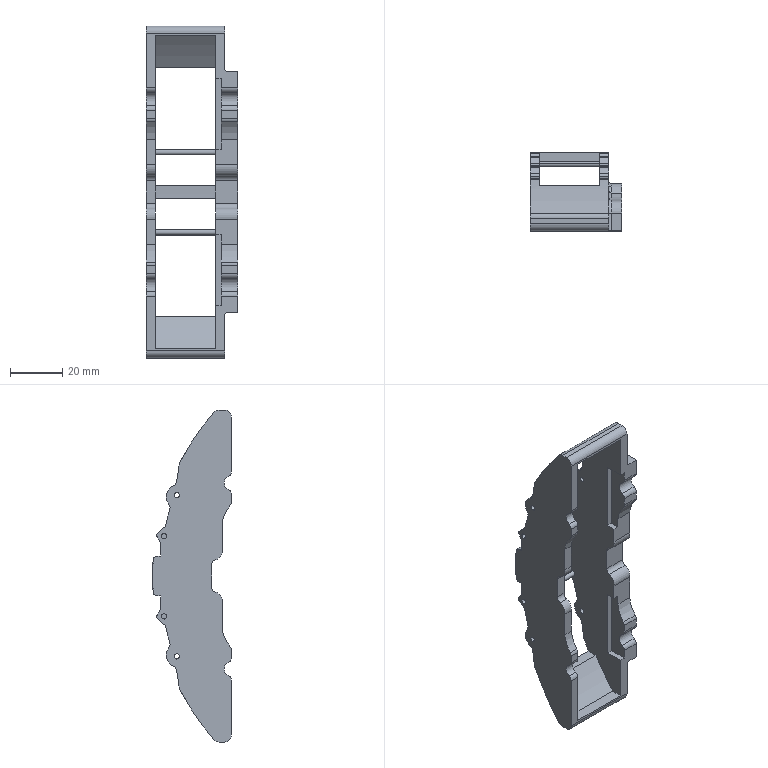Part | SolidWorks | features ICE 6, Fillet 2, Extrusion 1, Shell 1 | 1 solid | 179 faces | box 35 x 30 x 126.513 mm | volume 25595 mm3 | cylinder 107 | plane 63 | torus 8 | spline 1 | commonest cylinder face diameters 4 x36 2 x25 5.38 x8 9.085 x8 190 x7 5.437 x4